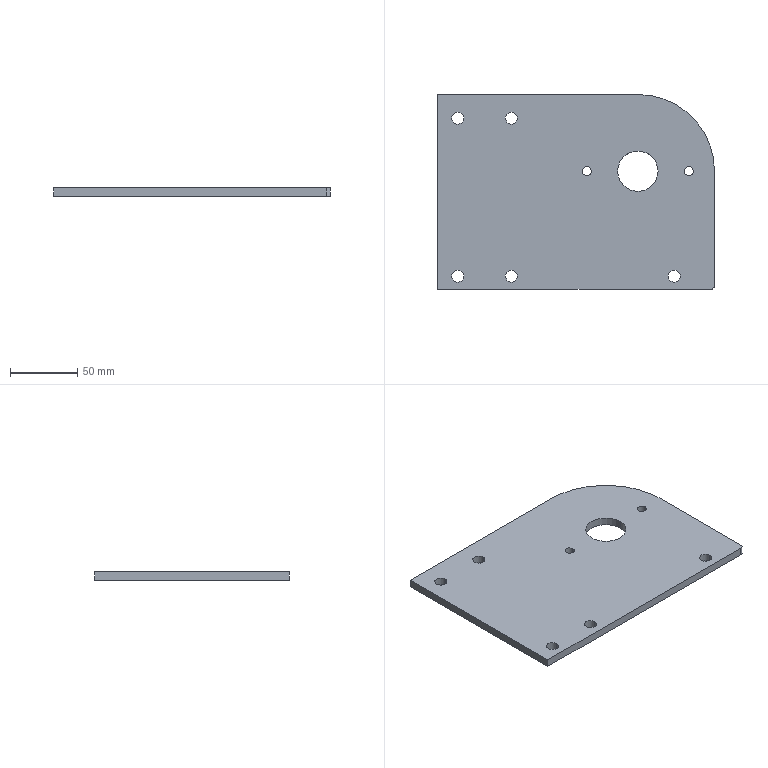Part | SolidWorks | features ICE 6, Fillet 5, HoleWzd 2, CirPattern 1, Extrusion 1 | 1 solid | 24 faces | box 206 x 145 x 6 mm | volume 168439 mm3 | cylinder 18 | plane 6 | commonest cylinder face diameters 9 x10 6.8 x4 30 x2 6 x1 114 x1
STEP:
#1=CARTESIAN_POINT('',(68.5,-62.5,0.));
#2=VERTEX_POINT('',#1);
#3=CARTESIAN_POINT('',(77.5,-62.5,0.));
#4=VERTEX_POINT('',#3);
#5=CARTESIAN_POINT('',(73.,-62.5,0.));
#6=DIRECTION('',(0.,0.,1.));
#7=DIRECTION('',(1.,0.,0.));
#8=AXIS2_PLACEMENT_3D('',#5,#6,#7);
#9=CIRCLE('',#8,4.5);
#10=EDGE_CURVE('',#2,#4,#9,.T.);
#11=ORIENTED_EDGE('',*,*,#10,.F.);
#12=CARTESIAN_POINT('',(68.5,-62.5,6.));
#13=VERTEX_POINT('',#12);
#14=CARTESIAN_POINT('',(68.5,-62.5,0.));
#15=DIRECTION('',(0.,0.,1.));
#16=VECTOR('',#15,1000.);
#17=LINE('',#14,#16);
#18=EDGE_CURVE('',#2,#13,#17,.T.);
#19=ORIENTED_EDGE('',*,*,#18,.T.);
#20=CARTESIAN_POINT('',(77.5,-62.5,6.));
#21=VERTEX_POINT('',#20);
#22=CARTESIAN_POINT('',(73.,-62.5,6.));
#23=DIRECTION('',(0.,0.,1.));
#24=DIRECTION('',(1.,0.,0.));
#25=AXIS2_PLACEMENT_3D('',#22,#23,#24);
#26=CIRCLE('',#25,4.5);
#27=EDGE_CURVE('',#13,#21,#26,.T.);
#28=ORIENTED_EDGE('',*,*,#27,.T.);
#29=CARTESIAN_POINT('',(77.5,-62.5,0.));
#30=DIRECTION('',(0.,0.,1.));
#31=VECTOR('',#30,1000.);
#32=LINE('',#29,#31);
#33=EDGE_CURVE('',#4,#21,#32,.T.);
#34=ORIENTED_EDGE('',*,*,#33,.F.);
#35=EDGE_LOOP('',(#11,#19,#28,#34));
#36=FACE_OUTER_BOUND('',#35,.T.);
#37=CARTESIAN_POINT('',(73.,-62.5,0.));
#38=DIRECTION('',(0.,0.,1.));
#39=DIRECTION('',(1.,0.,0.));
#40=AXIS2_PLACEMENT_3D('',#37,#38,#39);
#41=CYLINDRICAL_SURFACE('',#40,4.5);
#42=ADVANCED_FACE('',(#36),#41,.F.);
#43=CARTESIAN_POINT('',(80.6,15.5,0.));
#44=VERTEX_POINT('',#43);
#45=CARTESIAN_POINT('',(87.4,15.5,0.));
#46=VERTEX_POINT('',#45);
#47=CARTESIAN_POINT('',(84.,15.5,0.));
#48=DIRECTION('',(0.,0.,1.));
#49=DIRECTION('',(1.,0.,0.));
#50=AXIS2_PLACEMENT_3D('',#47,#48,#49);
#51=CIRCLE('',#50,3.4);
#52=EDGE_CURVE('',#44,#46,#51,.T.);
#53=ORIENTED_EDGE('',*,*,#52,.F.);
#54=CARTESIAN_POINT('',(80.6,15.5,6.));
#55=VERTEX_POINT('',#54);
#56=CARTESIAN_POINT('',(80.6,15.5,6.));
#57=DIRECTION('',(0.,0.,1.));
#58=VECTOR('',#57,1000.);
#59=LINE('',#56,#58);
#60=EDGE_CURVE('',#44,#55,#59,.T.);
#61=ORIENTED_EDGE('',*,*,#60,.T.);
#62=CARTESIAN_POINT('',(87.4,15.5,6.));
#63=VERTEX_POINT('',#62);
#64=CARTESIAN_POINT('',(84.,15.5,6.));
#65=DIRECTION('',(0.,0.,1.));
#66=DIRECTION('',(1.,0.,0.));
#67=AXIS2_PLACEMENT_3D('',#64,#65,#66);
#68=CIRCLE('',#67,3.4);
#69=EDGE_CURVE('',#55,#63,#68,.T.);
#70=ORIENTED_EDGE('',*,*,#69,.T.);
#71=CARTESIAN_POINT('',(87.4,15.5,6.));
#72=DIRECTION('',(0.,0.,1.));
#73=VECTOR('',#72,1000.);
#74=LINE('',#71,#73);
#75=EDGE_CURVE('',#46,#63,#74,.T.);
#76=ORIENTED_EDGE('',*,*,#75,.F.);
#77=EDGE_LOOP('',(#53,#61,#70,#76));
#78=FACE_OUTER_BOUND('',#77,.T.);
#79=CARTESIAN_POINT('',(84.,15.5,6.));
#80=DIRECTION('',(0.,0.,1.));
#81=DIRECTION('',(1.,0.,0.));
#82=AXIS2_PLACEMENT_3D('',#79,#80,#81);
#83=CYLINDRICAL_SURFACE('',#82,3.4);
#84=ADVANCED_FACE('',(#78),#83,.F.);
#85=CARTESIAN_POINT('',(4.6,15.5,0.));
#86=VERTEX_POINT('',#85);
#87=CARTESIAN_POINT('',(11.4,15.5,0.));
#88=VERTEX_POINT('',#87);
#89=CARTESIAN_POINT('',(8.,15.5,0.));
#90=DIRECTION('',(0.,0.,1.));
#91=DIRECTION('',(1.,0.,0.));
#92=AXIS2_PLACEMENT_3D('',#89,#90,#91);
#93=CIRCLE('',#92,3.4);
#94=EDGE_CURVE('',#86,#88,#93,.T.);
#95=ORIENTED_EDGE('',*,*,#94,.F.);
#96=CARTESIAN_POINT('',(4.6,15.5,6.));
#97=VERTEX_POINT('',#96);
#98=CARTESIAN_POINT('',(4.6,15.5,6.));
#99=DIRECTION('',(0.,0.,1.));
#100=VECTOR('',#99,1000.);
#101=LINE('',#98,#100);
#102=EDGE_CURVE('',#86,#97,#101,.T.);
#103=ORIENTED_EDGE('',*,*,#102,.T.);
#104=CARTESIAN_POINT('',(11.4,15.5,6.));
#105=VERTEX_POINT('',#104);
#106=CARTESIAN_POINT('',(8.,15.5,6.));
#107=DIRECTION('',(0.,0.,1.));
#108=DIRECTION('',(1.,0.,0.));
#109=AXIS2_PLACEMENT_3D('',#106,#107,#108);
#110=CIRCLE('',#109,3.4);
#111=EDGE_CURVE('',#97,#105,#110,.T.);
#112=ORIENTED_EDGE('',*,*,#111,.T.);
#113=CARTESIAN_POINT('',(11.4,15.5,6.));
#114=DIRECTION('',(0.,0.,1.));
#115=VECTOR('',#114,1000.);
#116=LINE('',#113,#115);
#117=EDGE_CURVE('',#88,#105,#116,.T.);
#118=ORIENTED_EDGE('',*,*,#117,.F.);
#119=EDGE_LOOP('',(#95,#103,#112,#118));
#120=FACE_OUTER_BOUND('',#119,.T.);
#121=CARTESIAN_POINT('',(8.,15.5,6.));
#122=DIRECTION('',(0.,0.,1.));
#123=DIRECTION('',(1.,0.,0.));
#124=AXIS2_PLACEMENT_3D('',#121,#122,#123);
#125=CYLINDRICAL_SURFACE('',#124,3.4);
#126=ADVANCED_FACE('',(#120),#125,.F.);
#127=CARTESIAN_POINT('',(31.,15.5,0.));
#128=VERTEX_POINT('',#127);
#129=CARTESIAN_POINT('',(61.,15.5,0.));
#130=VERTEX_POINT('',#129);
#131=CARTESIAN_POINT('',(46.,15.5,0.));
#132=DIRECTION('',(0.,0.,1.));
#133=DIRECTION('',(1.,0.,0.));
#134=AXIS2_PLACEMENT_3D('',#131,#132,#133);
#135=CIRCLE('',#134,15.);
#136=EDGE_CURVE('',#128,#130,#135,.T.);
#137=ORIENTED_EDGE('',*,*,#136,.F.);
#138=CARTESIAN_POINT('',(31.,15.5,6.));
#139=VERTEX_POINT('',#138);
#140=CARTESIAN_POINT('',(31.,15.5,0.));
#141=DIRECTION('',(0.,0.,1.));
#142=VECTOR('',#141,1000.);
#143=LINE('',#140,#142);
#144=EDGE_CURVE('',#128,#139,#143,.T.);
#145=ORIENTED_EDGE('',*,*,#144,.T.);
#146=CARTESIAN_POINT('',(61.,15.5,6.));
#147=VERTEX_POINT('',#146);
#148=CARTESIAN_POINT('',(46.,15.5,6.));
#149=DIRECTION('',(0.,0.,1.));
#150=DIRECTION('',(1.,0.,0.));
#151=AXIS2_PLACEMENT_3D('',#148,#149,#150);
#152=CIRCLE('',#151,15.);
#153=EDGE_CURVE('',#139,#147,#152,.T.);
#154=ORIENTED_EDGE('',*,*,#153,.T.);
#155=CARTESIAN_POINT('',(61.,15.5,0.));
#156=DIRECTION('',(0.,0.,1.));
#157=VECTOR('',#156,1000.);
#158=LINE('',#155,#157);
#159=EDGE_CURVE('',#130,#147,#158,.T.);
#160=ORIENTED_EDGE('',*,*,#159,.F.);
#161=EDGE_LOOP('',(#137,#145,#154,#160));
#162=FACE_OUTER_BOUND('',#161,.T.);
#163=CARTESIAN_POINT('',(46.,15.5,0.));
#164=DIRECTION('',(0.,0.,1.));
#165=DIRECTION('',(1.,0.,0.));
#166=AXIS2_PLACEMENT_3D('',#163,#164,#165);
#167=CYLINDRICAL_SURFACE('',#166,15.);
#168=ADVANCED_FACE('',(#162),#167,.F.);
#169=CARTESIAN_POINT('',(-52.5,-62.5,0.));
#170=VERTEX_POINT('',#169);
#171=CARTESIAN_POINT('',(-43.5,-62.5,0.));
#172=VERTEX_POINT('',#171);
#173=CARTESIAN_POINT('',(-48.,-62.5,0.));
#174=DIRECTION('',(0.,0.,1.));
#175=DIRECTION('',(1.,0.,0.));
#176=AXIS2_PLACEMENT_3D('',#173,#174,#175);
#177=CIRCLE('',#176,4.5);
#178=EDGE_CURVE('',#170,#172,#177,.T.);
#179=ORIENTED_EDGE('',*,*,#178,.F.);
#180=CARTESIAN_POINT('',(-52.5,-62.5,6.));
#181=VERTEX_POINT('',#180);
#182=CARTESIAN_POINT('',(-52.5,-62.5,0.));
#183=DIRECTION('',(0.,0.,1.));
#184=VECTOR('',#183,1000.);
#185=LINE('',#182,#184);
#186=EDGE_CURVE('',#170,#181,#185,.T.);
#187=ORIENTED_EDGE('',*,*,#186,.T.);
#188=CARTESIAN_POINT('',(-43.5,-62.5,6.));
#189=VERTEX_POINT('',#188);
#190=CARTESIAN_POINT('',(-48.,-62.5,6.));
#191=DIRECTION('',(0.,0.,1.));
#192=DIRECTION('',(1.,0.,0.));
#193=AXIS2_PLACEMENT_3D('',#190,#191,#192);
#194=CIRCLE('',#193,4.5);
#195=EDGE_CURVE('',#181,#189,#194,.T.);
#196=ORIENTED_EDGE('',*,*,#195,.T.);
#197=CARTESIAN_POINT('',(-43.5,-62.5,0.));
#198=DIRECTION('',(0.,0.,1.));
#199=VECTOR('',#198,1000.);
#200=LINE('',#197,#199);
#201=EDGE_CURVE('',#172,#189,#200,.T.);
#202=ORIENTED_EDGE('',*,*,#201,.F.);
#203=EDGE_LOOP('',(#179,#187,#196,#202));
#204=FACE_OUTER_BOUND('',#203,.T.);
#205=CARTESIAN_POINT('',(-48.,-62.5,0.));
#206=DIRECTION('',(0.,0.,1.));
#207=DIRECTION('',(1.,0.,0.));
#208=AXIS2_PLACEMENT_3D('',#205,#206,#207);
#209=CYLINDRICAL_SURFACE('',#208,4.5);
#210=ADVANCED_FACE('',(#204),#209,.F.);
#211=CARTESIAN_POINT('',(-92.5,-62.5,0.));
#212=VERTEX_POINT('',#211);
#213=CARTESIAN_POINT('',(-83.5,-62.5,0.));
#214=VERTEX_POINT('',#213);
#215=CARTESIAN_POINT('',(-88.,-62.5,0.));
#216=DIRECTION('',(0.,0.,1.));
#217=DIRECTION('',(1.,0.,0.));
#218=AXIS2_PLACEMENT_3D('',#215,#216,#217);
#219=CIRCLE('',#218,4.5);
#220=EDGE_CURVE('',#212,#214,#219,.T.);
#221=ORIENTED_EDGE('',*,*,#220,.F.);
#222=CARTESIAN_POINT('',(-92.5,-62.5,6.));
#223=VERTEX_POINT('',#222);
#224=CARTESIAN_POINT('',(-92.5,-62.5,0.));
#225=DIRECTION('',(0.,0.,1.));
#226=VECTOR('',#225,1000.);
#227=LINE('',#224,#226);
#228=EDGE_CURVE('',#212,#223,#227,.T.);
#229=ORIENTED_EDGE('',*,*,#228,.T.);
#230=CARTESIAN_POINT('',(-83.5,-62.5,6.));
#231=VERTEX_POINT('',#230);
#232=CARTESIAN_POINT('',(-88.,-62.5,6.));
#233=DIRECTION('',(0.,0.,1.));
#234=DIRECTION('',(1.,0.,0.));
#235=AXIS2_PLACEMENT_3D('',#232,#233,#234);
#236=CIRCLE('',#235,4.5);
#237=EDGE_CURVE('',#223,#231,#236,.T.);
#238=ORIENTED_EDGE('',*,*,#237,.T.);
#239=CARTESIAN_POINT('',(-83.5,-62.5,0.));
#240=DIRECTION('',(0.,0.,1.));
#241=VECTOR('',#240,1000.);
#242=LINE('',#239,#241);
#243=EDGE_CURVE('',#214,#231,#242,.T.);
#244=ORIENTED_EDGE('',*,*,#243,.F.);
#245=EDGE_LOOP('',(#221,#229,#238,#244));
#246=FACE_OUTER_BOUND('',#245,.T.);
#247=CARTESIAN_POINT('',(-88.,-62.5,0.));
#248=DIRECTION('',(0.,0.,1.));
#249=DIRECTION('',(1.,0.,0.));
#250=AXIS2_PLACEMENT_3D('',#247,#248,#249);
#251=CYLINDRICAL_SURFACE('',#250,4.5);
#252=ADVANCED_FACE('',(#246),#251,.F.);
#253=CARTESIAN_POINT('',(-52.5,55.,0.));
#254=VERTEX_POINT('',#253);
#255=CARTESIAN_POINT('',(-43.5,55.,0.));
#256=VERTEX_POINT('',#255);
#257=CARTESIAN_POINT('',(-48.,55.,0.));
#258=DIRECTION('',(0.,0.,1.));
#259=DIRECTION('',(1.,0.,0.));
#260=AXIS2_PLACEMENT_3D('',#257,#258,#259);
#261=CIRCLE('',#260,4.5);
#262=EDGE_CURVE('',#254,#256,#261,.T.);
#263=ORIENTED_EDGE('',*,*,#262,.F.);
#264=CARTESIAN_POINT('',(-52.5,55.,6.));
#265=VERTEX_POINT('',#264);
#266=CARTESIAN_POINT('',(-52.5,55.,0.));
#267=DIRECTION('',(0.,0.,1.));
#268=VECTOR('',#267,1000.);
#269=LINE('',#266,#268);
#270=EDGE_CURVE('',#254,#265,#269,.T.);
#271=ORIENTED_EDGE('',*,*,#270,.T.);
#272=CARTESIAN_POINT('',(-43.5,55.,6.));
#273=VERTEX_POINT('',#272);
#274=CARTESIAN_POINT('',(-48.,55.,6.));
#275=DIRECTION('',(0.,0.,1.));
#276=DIRECTION('',(1.,0.,0.));
#277=AXIS2_PLACEMENT_3D('',#274,#275,#276);
#278=CIRCLE('',#277,4.5);
#279=EDGE_CURVE('',#265,#273,#278,.T.);
#280=ORIENTED_EDGE('',*,*,#279,.T.);
#281=CARTESIAN_POINT('',(-43.5,55.,0.));
#282=DIRECTION('',(0.,0.,1.));
#283=VECTOR('',#282,1000.);
#284=LINE('',#281,#283);
#285=EDGE_CURVE('',#256,#273,#284,.T.);
#286=ORIENTED_EDGE('',*,*,#285,.F.);
#287=EDGE_LOOP('',(#263,#271,#280,#286));
#288=FACE_OUTER_BOUND('',#287,.T.);
#289=CARTESIAN_POINT('',(-48.,55.,0.));
#290=DIRECTION('',(0.,0.,1.));
#291=DIRECTION('',(1.,0.,0.));
#292=AXIS2_PLACEMENT_3D('',#289,#290,#291);
#293=CYLINDRICAL_SURFACE('',#292,4.5);
#294=ADVANCED_FACE('',(#288),#293,.F.);
#295=CARTESIAN_POINT('',(-92.5,55.,0.));
#296=VERTEX_POINT('',#295);
#297=CARTESIAN_POINT('',(-83.5,55.,0.));
#298=VERTEX_POINT('',#297);
#299=CARTESIAN_POINT('',(-88.,55.,0.));
#300=DIRECTION('',(0.,0.,1.));
#301=DIRECTION('',(1.,0.,0.));
#302=AXIS2_PLACEMENT_3D('',#299,#300,#301);
#303=CIRCLE('',#302,4.5);
#304=EDGE_CURVE('',#296,#298,#303,.T.);
#305=ORIENTED_EDGE('',*,*,#304,.F.);
#306=CARTESIAN_POINT('',(-92.5,55.,6.));
#307=VERTEX_POINT('',#306);
#308=CARTESIAN_POINT('',(-92.5,55.,0.));
#309=DIRECTION('',(0.,0.,1.));
#310=VECTOR('',#309,1000.);
#311=LINE('',#308,#310);
#312=EDGE_CURVE('',#296,#307,#311,.T.);
#313=ORIENTED_EDGE('',*,*,#312,.T.);
#314=CARTESIAN_POINT('',(-83.5,55.,6.));
#315=VERTEX_POINT('',#314);
#316=CARTESIAN_POINT('',(-88.,55.,6.));
#317=DIRECTION('',(0.,0.,1.));
#318=DIRECTION('',(1.,0.,0.));
#319=AXIS2_PLACEMENT_3D('',#316,#317,#318);
#320=CIRCLE('',#319,4.5);
#321=EDGE_CURVE('',#307,#315,#320,.T.);
#322=ORIENTED_EDGE('',*,*,#321,.T.);
#323=CARTESIAN_POINT('',(-83.5,55.,0.));
#324=DIRECTION('',(0.,0.,1.));
#325=VECTOR('',#324,1000.);
#326=LINE('',#323,#325);
#327=EDGE_CURVE('',#298,#315,#326,.T.);
#328=ORIENTED_EDGE('',*,*,#327,.F.);
#329=EDGE_LOOP('',(#305,#313,#322,#328));
#330=FACE_OUTER_BOUND('',#329,.T.);
#331=CARTESIAN_POINT('',(-88.,55.,0.));
#332=DIRECTION('',(0.,0.,1.));
#333=DIRECTION('',(1.,0.,0.));
#334=AXIS2_PLACEMENT_3D('',#331,#332,#333);
#335=CYLINDRICAL_SURFACE('',#334,4.5);
#336=ADVANCED_FACE('',(#330),#335,.F.);
#337=CARTESIAN_POINT('',(-103.,72.5,0.));
#338=VERTEX_POINT('',#337);
#339=CARTESIAN_POINT('',(-103.,-72.5,0.));
#340=VERTEX_POINT('',#339);
#341=CARTESIAN_POINT('',(-103.,72.5,0.));
#342=DIRECTION('',(0.,-1.,0.));
#343=VECTOR('',#342,1000.);
#344=LINE('',#341,#343);
#345=EDGE_CURVE('',#338,#340,#344,.T.);
#346=ORIENTED_EDGE('',*,*,#345,.T.);
#347=CARTESIAN_POINT('',(-103.,-72.5,6.));
#348=VERTEX_POINT('',#347);
#349=CARTESIAN_POINT('',(-103.,-72.5,6.));
#350=DIRECTION('',(0.,0.,-1.));
#351=VECTOR('',#350,1000.);
#352=LINE('',#349,#351);
#353=EDGE_CURVE('',#348,#340,#352,.T.);
#354=ORIENTED_EDGE('',*,*,#353,.F.);
#355=CARTESIAN_POINT('',(-103.,72.5,6.));
#356=VERTEX_POINT('',#355);
#357=CARTESIAN_POINT('',(-103.,72.5,6.));
#358=DIRECTION('',(0.,-1.,0.));
#359=VECTOR('',#358,1000.);
#360=LINE('',#357,#359);
#361=EDGE_CURVE('',#356,#348,#360,.T.);
#362=ORIENTED_EDGE('',*,*,#361,.F.);
#363=CARTESIAN_POINT('',(-103.,72.5,6.));
#364=DIRECTION('',(0.,0.,-1.));
#365=VECTOR('',#364,1000.);
#366=LINE('',#363,#365);
#367=EDGE_CURVE('',#356,#338,#366,.T.);
#368=ORIENTED_EDGE('',*,*,#367,.T.);
#369=EDGE_LOOP('',(#346,#354,#362,#368));
#370=FACE_OUTER_BOUND('',#369,.T.);
#371=CARTESIAN_POINT('',(-103.,72.5,6.));
#372=DIRECTION('',(1.,0.,0.));
#373=DIRECTION('',(0.,0.,-1.));
#374=AXIS2_PLACEMENT_3D('',#371,#372,#373);
#375=PLANE('',#374);
#376=ADVANCED_FACE('',(#370),#375,.F.);
#377=CARTESIAN_POINT('',(100.,-72.5,0.));
#378=VERTEX_POINT('',#377);
#379=CARTESIAN_POINT('',(-103.,-72.5,0.));
#380=DIRECTION('',(1.,0.,0.));
#381=VECTOR('',#380,1000.);
#382=LINE('',#379,#381);
#383=EDGE_CURVE('',#340,#378,#382,.T.);
#384=ORIENTED_EDGE('',*,*,#383,.T.);
#385=CARTESIAN_POINT('',(100.,-72.5,6.));
#386=VERTEX_POINT('',#385);
#387=CARTESIAN_POINT('',(100.,-72.5,6.));
#388=DIRECTION('',(0.,0.,1.));
#389=VECTOR('',#388,1000.);
#390=LINE('',#387,#389);
#391=EDGE_CURVE('',#378,#386,#390,.T.);
#392=ORIENTED_EDGE('',*,*,#391,.T.);
#393=CARTESIAN_POINT('',(-103.,-72.5,6.));
#394=DIRECTION('',(1.,0.,0.));
#395=VECTOR('',#394,1000.);
#396=LINE('',#393,#395);
#397=EDGE_CURVE('',#348,#386,#396,.T.);
#398=ORIENTED_EDGE('',*,*,#397,.F.);
#399=ORIENTED_EDGE('',*,*,#353,.T.);
#400=EDGE_LOOP('',(#384,#392,#398,#399));
#401=FACE_OUTER_BOUND('',#400,.T.);
#402=CARTESIAN_POINT('',(-103.,-72.5,6.));
#403=DIRECTION('',(0.,1.,0.));
#404=DIRECTION('',(0.,0.,1.));
#405=AXIS2_PLACEMENT_3D('',#402,#403,#404);
#406=PLANE('',#405);
#407=ADVANCED_FACE('',(#401),#406,.F.);
#408=CARTESIAN_POINT('',(103.,-69.5,6.));
#409=VERTEX_POINT('',#408);
#410=CARTESIAN_POINT('',(103.,15.5,6.));
#411=VERTEX_POINT('',#410);
#412=CARTESIAN_POINT('',(103.,72.5,6.));
#413=DIRECTION('',(0.,1.,0.));
#414=VECTOR('',#413,1000.);
#415=LINE('',#412,#414);
#416=EDGE_CURVE('',#409,#411,#415,.T.);
#417=ORIENTED_EDGE('',*,*,#416,.F.);
#418=CARTESIAN_POINT('',(103.,-69.5,0.));
#419=VERTEX_POINT('',#418);
#420=CARTESIAN_POINT('',(103.,-69.5,6.));
#421=DIRECTION('',(0.,0.,-1.));
#422=VECTOR('',#421,1000.);
#423=LINE('',#420,#422);
#424=EDGE_CURVE('',#409,#419,#423,.T.);
#425=ORIENTED_EDGE('',*,*,#424,.T.);
#426=CARTESIAN_POINT('',(103.,15.5,0.));
#427=VERTEX_POINT('',#426);
#428=CARTESIAN_POINT('',(103.,72.5,0.));
#429=DIRECTION('',(0.,1.,0.));
#430=VECTOR('',#429,1000.);
#431=LINE('',#428,#430);
#432=EDGE_CURVE('',#419,#427,#431,.T.);
#433=ORIENTED_EDGE('',*,*,#432,.T.);
#434=CARTESIAN_POINT('',(103.,15.5,6.));
#435=DIRECTION('',(0.,0.,1.));
#436=VECTOR('',#435,1000.);
#437=LINE('',#434,#436);
#438=EDGE_CURVE('',#427,#411,#437,.T.);
#439=ORIENTED_EDGE('',*,*,#438,.T.);
#440=EDGE_LOOP('',(#417,#425,#433,#439));
#441=FACE_OUTER_BOUND('',#440,.T.);
#442=CARTESIAN_POINT('',(103.,72.5,6.));
#443=DIRECTION('',(-1.,0.,0.));
#444=DIRECTION('',(0.,0.,1.));
#445=AXIS2_PLACEMENT_3D('',#442,#443,#444);
#446=PLANE('',#445);
#447=ADVANCED_FACE('',(#441),#446,.F.);
#448=CARTESIAN_POINT('',(46.,72.5,6.));
#449=VERTEX_POINT('',#448);
#450=CARTESIAN_POINT('',(-103.,72.5,6.));
#451=DIRECTION('',(-1.,0.,0.));
#452=VECTOR('',#451,1000.);
#453=LINE('',#450,#452);
#454=EDGE_CURVE('',#449,#356,#453,.T.);
#455=ORIENTED_EDGE('',*,*,#454,.F.);
#456=CARTESIAN_POINT('',(46.,72.5,0.));
#457=VERTEX_POINT('',#456);
#458=CARTESIAN_POINT('',(46.,72.5,6.));
#459=DIRECTION('',(0.,0.,-1.));
#460=VECTOR('',#459,1000.);
#461=LINE('',#458,#460);
#462=EDGE_CURVE('',#449,#457,#461,.T.);
#463=ORIENTED_EDGE('',*,*,#462,.T.);
#464=CARTESIAN_POINT('',(-103.,72.5,0.));
#465=DIRECTION('',(-1.,0.,0.));
#466=VECTOR('',#465,1000.);
#467=LINE('',#464,#466);
#468=EDGE_CURVE('',#457,#338,#467,.T.);
#469=ORIENTED_EDGE('',*,*,#468,.T.);
#470=ORIENTED_EDGE('',*,*,#367,.F.);
#471=EDGE_LOOP('',(#455,#463,#469,#470));
#472=FACE_OUTER_BOUND('',#471,.T.);
#473=CARTESIAN_POINT('',(-103.,72.5,6.));
#474=DIRECTION('',(0.,-1.,0.));
#475=DIRECTION('',(0.,0.,-1.));
#476=AXIS2_PLACEMENT_3D('',#473,#474,#475);
#477=PLANE('',#476);
#478=ADVANCED_FACE('',(#472),#477,.F.);
#479=CARTESIAN_POINT('',(73.,-62.5,6.));
#480=DIRECTION('',(0.,0.,1.));
#481=DIRECTION('',(1.,0.,0.));
#482=AXIS2_PLACEMENT_3D('',#479,#480,#481);
#483=CIRCLE('',#482,4.5);
#484=EDGE_CURVE('',#21,#13,#483,.T.);
#485=ORIENTED_EDGE('',*,*,#484,.F.);
#486=ORIENTED_EDGE('',*,*,#27,.F.);
#487=EDGE_LOOP('',(#485,#486));
#488=FACE_BOUND('',#487,.T.);
#489=CARTESIAN_POINT('',(84.,15.5,6.));
#490=DIRECTION('',(0.,0.,1.));
#491=DIRECTION('',(1.,0.,0.));
#492=AXIS2_PLACEMENT_3D('',#489,#490,#491);
#493=CIRCLE('',#492,3.4);
#494=EDGE_CURVE('',#63,#55,#493,.T.);
#495=ORIENTED_EDGE('',*,*,#494,.F.);
#496=ORIENTED_EDGE('',*,*,#69,.F.);
#497=EDGE_LOOP('',(#495,#496));
#498=FACE_BOUND('',#497,.T.);
#499=CARTESIAN_POINT('',(8.,15.5,6.));
#500=DIRECTION('',(0.,0.,1.));
#501=DIRECTION('',(1.,0.,0.));
#502=AXIS2_PLACEMENT_3D('',#499,#500,#501);
#503=CIRCLE('',#502,3.4);
#504=EDGE_CURVE('',#105,#97,#503,.T.);
#505=ORIENTED_EDGE('',*,*,#504,.F.);
#506=ORIENTED_EDGE('',*,*,#111,.F.);
#507=EDGE_LOOP('',(#505,#506));
#508=FACE_BOUND('',#507,.T.);
#509=CARTESIAN_POINT('',(46.,15.5,6.));
#510=DIRECTION('',(0.,0.,1.));
#511=DIRECTION('',(1.,0.,0.));
#512=AXIS2_PLACEMENT_3D('',#509,#510,#511);
#513=CIRCLE('',#512,15.);
#514=EDGE_CURVE('',#147,#139,#513,.T.);
#515=ORIENTED_EDGE('',*,*,#514,.F.);
#516=ORIENTED_EDGE('',*,*,#153,.F.);
#517=EDGE_LOOP('',(#515,#516));
#518=FACE_BOUND('',#517,.T.);
#519=CARTESIAN_POINT('',(-48.,-62.5,6.));
#520=DIRECTION('',(0.,0.,1.));
#521=DIRECTION('',(1.,0.,0.));
#522=AXIS2_PLACEMENT_3D('',#519,#520,#521);
#523=CIRCLE('',#522,4.5);
#524=EDGE_CURVE('',#189,#181,#523,.T.);
#525=ORIENTED_EDGE('',*,*,#524,.F.);
#526=ORIENTED_EDGE('',*,*,#195,.F.);
#527=EDGE_LOOP('',(#525,#526));
#528=FACE_BOUND('',#527,.T.);
#529=CARTESIAN_POINT('',(-88.,-62.5,6.));
#530=DIRECTION('',(0.,0.,1.));
#531=DIRECTION('',(1.,0.,0.));
#532=AXIS2_PLACEMENT_3D('',#529,#530,#531);
#533=CIRCLE('',#532,4.5);
#534=EDGE_CURVE('',#231,#223,#533,.T.);
#535=ORIENTED_EDGE('',*,*,#534,.F.);
#536=ORIENTED_EDGE('',*,*,#237,.F.);
#537=EDGE_LOOP('',(#535,#536));
#538=FACE_BOUND('',#537,.T.);
#539=CARTESIAN_POINT('',(-48.,55.,6.));
#540=DIRECTION('',(0.,0.,1.));
#541=DIRECTION('',(1.,0.,0.));
#542=AXIS2_PLACEMENT_3D('',#539,#540,#541);
#543=CIRCLE('',#542,4.5);
#544=EDGE_CURVE('',#273,#265,#543,.T.);
#545=ORIENTED_EDGE('',*,*,#544,.F.);
#546=ORIENTED_EDGE('',*,*,#279,.F.);
#547=EDGE_LOOP('',(#545,#546));
#548=FACE_BOUND('',#547,.T.);
#549=CARTESIAN_POINT('',(-88.,55.,6.));
#550=DIRECTION('',(0.,0.,1.));
#551=DIRECTION('',(1.,0.,0.));
#552=AXIS2_PLACEMENT_3D('',#549,#550,#551);
#553=CIRCLE('',#552,4.5);
#554=EDGE_CURVE('',#315,#307,#553,.T.);
#555=ORIENTED_EDGE('',*,*,#554,.F.);
#556=ORIENTED_EDGE('',*,*,#321,.F.);
#557=EDGE_LOOP('',(#555,#556));
#558=FACE_BOUND('',#557,.T.);
#559=ORIENTED_EDGE('',*,*,#397,.T.);
#560=CARTESIAN_POINT('',(100.,-69.5,6.));
#561=DIRECTION('',(0.,0.,1.));
#562=DIRECTION('',(1.,0.,0.));
#563=AXIS2_PLACEMENT_3D('',#560,#561,#562);
#564=CIRCLE('',#563,3.);
#565=EDGE_CURVE('',#386,#409,#564,.T.);
#566=ORIENTED_EDGE('',*,*,#565,.T.);
#567=ORIENTED_EDGE('',*,*,#416,.T.);
#568=CARTESIAN_POINT('',(46.,15.5,6.));
#569=DIRECTION('',(0.,0.,1.));
#570=DIRECTION('',(1.,0.,0.));
#571=AXIS2_PLACEMENT_3D('',#568,#569,#570);
#572=CIRCLE('',#571,57.);
#573=EDGE_CURVE('',#411,#449,#572,.T.);
#574=ORIENTED_EDGE('',*,*,#573,.T.);
#575=ORIENTED_EDGE('',*,*,#454,.T.);
#576=ORIENTED_EDGE('',*,*,#361,.T.);
#577=EDGE_LOOP('',(#559,#566,#567,#574,#575,#576));
#578=FACE_OUTER_BOUND('',#577,.T.);
#579=CARTESIAN_POINT('',(0.,0.,6.));
#580=DIRECTION('',(0.,0.,1.));
#581=DIRECTION('',(1.,0.,0.));
#582=AXIS2_PLACEMENT_3D('',#579,#580,#581);
#583=PLANE('',#582);
#584=ADVANCED_FACE('',(#488,#498,#508,#518,#528,#538,#548,#558,#578),#583,.T.);
#585=CARTESIAN_POINT('',(73.,-62.5,0.));
#586=DIRECTION('',(0.,0.,1.));
#587=DIRECTION('',(1.,0.,0.));
#588=AXIS2_PLACEMENT_3D('',#585,#586,#587);
#589=CIRCLE('',#588,4.5);
#590=EDGE_CURVE('',#4,#2,#589,.T.);
#591=ORIENTED_EDGE('',*,*,#590,.T.);
#592=ORIENTED_EDGE('',*,*,#10,.T.);
#593=EDGE_LOOP('',(#591,#592));
#594=FACE_BOUND('',#593,.T.);
#595=CARTESIAN_POINT('',(84.,15.5,0.));
#596=DIRECTION('',(0.,0.,1.));
#597=DIRECTION('',(1.,0.,0.));
#598=AXIS2_PLACEMENT_3D('',#595,#596,#597);
#599=CIRCLE('',#598,3.4);
#600=EDGE_CURVE('',#46,#44,#599,.T.);
#601=ORIENTED_EDGE('',*,*,#600,.T.);
#602=ORIENTED_EDGE('',*,*,#52,.T.);
#603=EDGE_LOOP('',(#601,#602));
#604=FACE_BOUND('',#603,.T.);
#605=CARTESIAN_POINT('',(8.,15.5,0.));
#606=DIRECTION('',(0.,0.,1.));
#607=DIRECTION('',(1.,0.,0.));
#608=AXIS2_PLACEMENT_3D('',#605,#606,#607);
#609=CIRCLE('',#608,3.4);
#610=EDGE_CURVE('',#88,#86,#609,.T.);
#611=ORIENTED_EDGE('',*,*,#610,.T.);
#612=ORIENTED_EDGE('',*,*,#94,.T.);
#613=EDGE_LOOP('',(#611,#612));
#614=FACE_BOUND('',#613,.T.);
#615=CARTESIAN_POINT('',(46.,15.5,0.));
#616=DIRECTION('',(0.,0.,1.));
#617=DIRECTION('',(1.,0.,0.));
#618=AXIS2_PLACEMENT_3D('',#615,#616,#617);
#619=CIRCLE('',#618,15.);
#620=EDGE_CURVE('',#130,#128,#619,.T.);
#621=ORIENTED_EDGE('',*,*,#620,.T.);
#622=ORIENTED_EDGE('',*,*,#136,.T.);
#623=EDGE_LOOP('',(#621,#622));
#624=FACE_BOUND('',#623,.T.);
#625=CARTESIAN_POINT('',(-48.,-62.5,0.));
#626=DIRECTION('',(0.,0.,1.));
#627=DIRECTION('',(1.,0.,0.));
#628=AXIS2_PLACEMENT_3D('',#625,#626,#627);
#629=CIRCLE('',#628,4.5);
#630=EDGE_CURVE('',#172,#170,#629,.T.);
#631=ORIENTED_EDGE('',*,*,#630,.T.);
#632=ORIENTED_EDGE('',*,*,#178,.T.);
#633=EDGE_LOOP('',(#631,#632));
#634=FACE_BOUND('',#633,.T.);
#635=CARTESIAN_POINT('',(-88.,-62.5,0.));
#636=DIRECTION('',(0.,0.,1.));
#637=DIRECTION('',(1.,0.,0.));
#638=AXIS2_PLACEMENT_3D('',#635,#636,#637);
#639=CIRCLE('',#638,4.5);
#640=EDGE_CURVE('',#214,#212,#639,.T.);
#641=ORIENTED_EDGE('',*,*,#640,.T.);
#642=ORIENTED_EDGE('',*,*,#220,.T.);
#643=EDGE_LOOP('',(#641,#642));
#644=FACE_BOUND('',#643,.T.);
#645=CARTESIAN_POINT('',(-48.,55.,0.));
#646=DIRECTION('',(0.,0.,1.));
#647=DIRECTION('',(1.,0.,0.));
#648=AXIS2_PLACEMENT_3D('',#645,#646,#647);
#649=CIRCLE('',#648,4.5);
#650=EDGE_CURVE('',#256,#254,#649,.T.);
#651=ORIENTED_EDGE('',*,*,#650,.T.);
#652=ORIENTED_EDGE('',*,*,#262,.T.);
#653=EDGE_LOOP('',(#651,#652));
#654=FACE_BOUND('',#653,.T.);
#655=CARTESIAN_POINT('',(-88.,55.,0.));
#656=DIRECTION('',(0.,0.,1.));
#657=DIRECTION('',(1.,0.,0.));
#658=AXIS2_PLACEMENT_3D('',#655,#656,#657);
#659=CIRCLE('',#658,4.5);
#660=EDGE_CURVE('',#298,#296,#659,.T.);
#661=ORIENTED_EDGE('',*,*,#660,.T.);
#662=ORIENTED_EDGE('',*,*,#304,.T.);
#663=EDGE_LOOP('',(#661,#662));
#664=FACE_BOUND('',#663,.T.);
#665=ORIENTED_EDGE('',*,*,#432,.F.);
#666=CARTESIAN_POINT('',(100.,-69.5,0.));
#667=DIRECTION('',(0.,0.,-1.));
#668=DIRECTION('',(1.,0.,0.));
#669=AXIS2_PLACEMENT_3D('',#666,#667,#668);
#670=CIRCLE('',#669,3.);
#671=EDGE_CURVE('',#419,#378,#670,.T.);
#672=ORIENTED_EDGE('',*,*,#671,.T.);
#673=ORIENTED_EDGE('',*,*,#383,.F.);
#674=ORIENTED_EDGE('',*,*,#345,.F.);
#675=ORIENTED_EDGE('',*,*,#468,.F.);
#676=CARTESIAN_POINT('',(46.,15.5,0.));
#677=DIRECTION('',(0.,0.,-1.));
#678=DIRECTION('',(1.,0.,0.));
#679=AXIS2_PLACEMENT_3D('',#676,#677,#678);
#680=CIRCLE('',#679,57.);
#681=EDGE_CURVE('',#457,#427,#680,.T.);
#682=ORIENTED_EDGE('',*,*,#681,.T.);
#683=EDGE_LOOP('',(#665,#672,#673,#674,#675,#682));
#684=FACE_OUTER_BOUND('',#683,.T.);
#685=CARTESIAN_POINT('',(0.,0.,0.));
#686=DIRECTION('',(0.,0.,1.));
#687=DIRECTION('',(1.,0.,0.));
#688=AXIS2_PLACEMENT_3D('',#685,#686,#687);
#689=PLANE('',#688);
#690=ADVANCED_FACE('',(#594,#604,#614,#624,#634,#644,#654,#664,#684),#689,.F.);
#691=ORIENTED_EDGE('',*,*,#312,.F.);
#692=ORIENTED_EDGE('',*,*,#660,.F.);
#693=ORIENTED_EDGE('',*,*,#327,.T.);
#694=ORIENTED_EDGE('',*,*,#554,.T.);
#695=EDGE_LOOP('',(#691,#692,#693,#694));
#696=FACE_OUTER_BOUND('',#695,.T.);
#697=CARTESIAN_POINT('',(-88.,55.,0.));
#698=DIRECTION('',(0.,0.,1.));
#699=DIRECTION('',(1.,0.,0.));
#700=AXIS2_PLACEMENT_3D('',#697,#698,#699);
#701=CYLINDRICAL_SURFACE('',#700,4.5);
#702=ADVANCED_FACE('',(#696),#701,.F.);
#703=ORIENTED_EDGE('',*,*,#270,.F.);
#704=ORIENTED_EDGE('',*,*,#650,.F.);
#705=ORIENTED_EDGE('',*,*,#285,.T.);
#706=ORIENTED_EDGE('',*,*,#544,.T.);
#707=EDGE_LOOP('',(#703,#704,#705,#706));
#708=FACE_OUTER_BOUND('',#707,.T.);
#709=CARTESIAN_POINT('',(-48.,55.,0.));
#710=DIRECTION('',(0.,0.,1.));
#711=DIRECTION('',(1.,0.,0.));
#712=AXIS2_PLACEMENT_3D('',#709,#710,#711);
#713=CYLINDRICAL_SURFACE('',#712,4.5);
#714=ADVANCED_FACE('',(#708),#713,.F.);
#715=ORIENTED_EDGE('',*,*,#228,.F.);
#716=ORIENTED_EDGE('',*,*,#640,.F.);
#717=ORIENTED_EDGE('',*,*,#243,.T.);
#718=ORIENTED_EDGE('',*,*,#534,.T.);
#719=EDGE_LOOP('',(#715,#716,#717,#718));
#720=FACE_OUTER_BOUND('',#719,.T.);
#721=CARTESIAN_POINT('',(-88.,-62.5,0.));
#722=DIRECTION('',(0.,0.,1.));
#723=DIRECTION('',(1.,0.,0.));
#724=AXIS2_PLACEMENT_3D('',#721,#722,#723);
#725=CYLINDRICAL_SURFACE('',#724,4.5);
#726=ADVANCED_FACE('',(#720),#725,.F.);
#727=ORIENTED_EDGE('',*,*,#186,.F.);
#728=ORIENTED_EDGE('',*,*,#630,.F.);
#729=ORIENTED_EDGE('',*,*,#201,.T.);
#730=ORIENTED_EDGE('',*,*,#524,.T.);
#731=EDGE_LOOP('',(#727,#728,#729,#730));
#732=FACE_OUTER_BOUND('',#731,.T.);
#733=CARTESIAN_POINT('',(-48.,-62.5,0.));
#734=DIRECTION('',(0.,0.,1.));
#735=DIRECTION('',(1.,0.,0.));
#736=AXIS2_PLACEMENT_3D('',#733,#734,#735);
#737=CYLINDRICAL_SURFACE('',#736,4.5);
#738=ADVANCED_FACE('',(#732),#737,.F.);
#739=ORIENTED_EDGE('',*,*,#144,.F.);
#740=ORIENTED_EDGE('',*,*,#620,.F.);
#741=ORIENTED_EDGE('',*,*,#159,.T.);
#742=ORIENTED_EDGE('',*,*,#514,.T.);
#743=EDGE_LOOP('',(#739,#740,#741,#742));
#744=FACE_OUTER_BOUND('',#743,.T.);
#745=CARTESIAN_POINT('',(46.,15.5,0.));
#746=DIRECTION('',(0.,0.,1.));
#747=DIRECTION('',(1.,0.,0.));
#748=AXIS2_PLACEMENT_3D('',#745,#746,#747);
#749=CYLINDRICAL_SURFACE('',#748,15.);
#750=ADVANCED_FACE('',(#744),#749,.F.);
#751=ORIENTED_EDGE('',*,*,#573,.F.);
#752=ORIENTED_EDGE('',*,*,#438,.F.);
#753=ORIENTED_EDGE('',*,*,#681,.F.);
#754=ORIENTED_EDGE('',*,*,#462,.F.);
#755=EDGE_LOOP('',(#751,#752,#753,#754));
#756=FACE_OUTER_BOUND('',#755,.T.);
#757=CARTESIAN_POINT('',(46.,15.5,6.));
#758=DIRECTION('',(0.,0.,-1.));
#759=DIRECTION('',(-1.,0.,0.));
#760=AXIS2_PLACEMENT_3D('',#757,#758,#759);
#761=CYLINDRICAL_SURFACE('',#760,57.);
#762=ADVANCED_FACE('',(#756),#761,.T.);
#763=ORIENTED_EDGE('',*,*,#102,.F.);
#764=ORIENTED_EDGE('',*,*,#610,.F.);
#765=ORIENTED_EDGE('',*,*,#117,.T.);
#766=ORIENTED_EDGE('',*,*,#504,.T.);
#767=EDGE_LOOP('',(#763,#764,#765,#766));
#768=FACE_OUTER_BOUND('',#767,.T.);
#769=CARTESIAN_POINT('',(8.,15.5,6.));
#770=DIRECTION('',(0.,0.,1.));
#771=DIRECTION('',(1.,0.,0.));
#772=AXIS2_PLACEMENT_3D('',#769,#770,#771);
#773=CYLINDRICAL_SURFACE('',#772,3.4);
#774=ADVANCED_FACE('',(#768),#773,.F.);
#775=ORIENTED_EDGE('',*,*,#60,.F.);
#776=ORIENTED_EDGE('',*,*,#600,.F.);
#777=ORIENTED_EDGE('',*,*,#75,.T.);
#778=ORIENTED_EDGE('',*,*,#494,.T.);
#779=EDGE_LOOP('',(#775,#776,#777,#778));
#780=FACE_OUTER_BOUND('',#779,.T.);
#781=CARTESIAN_POINT('',(84.,15.5,6.));
#782=DIRECTION('',(0.,0.,1.));
#783=DIRECTION('',(1.,0.,0.));
#784=AXIS2_PLACEMENT_3D('',#781,#782,#783);
#785=CYLINDRICAL_SURFACE('',#784,3.4);
#786=ADVANCED_FACE('',(#780),#785,.F.);
#787=ORIENTED_EDGE('',*,*,#18,.F.);
#788=ORIENTED_EDGE('',*,*,#590,.F.);
#789=ORIENTED_EDGE('',*,*,#33,.T.);
#790=ORIENTED_EDGE('',*,*,#484,.T.);
#791=EDGE_LOOP('',(#787,#788,#789,#790));
#792=FACE_OUTER_BOUND('',#791,.T.);
#793=CARTESIAN_POINT('',(73.,-62.5,0.));
#794=DIRECTION('',(0.,0.,1.));
#795=DIRECTION('',(1.,0.,0.));
#796=AXIS2_PLACEMENT_3D('',#793,#794,#795);
#797=CYLINDRICAL_SURFACE('',#796,4.5);
#798=ADVANCED_FACE('',(#792),#797,.F.);
#799=ORIENTED_EDGE('',*,*,#565,.F.);
#800=ORIENTED_EDGE('',*,*,#391,.F.);
#801=ORIENTED_EDGE('',*,*,#671,.F.);
#802=ORIENTED_EDGE('',*,*,#424,.F.);
#803=EDGE_LOOP('',(#799,#800,#801,#802));
#804=FACE_OUTER_BOUND('',#803,.T.);
#805=CARTESIAN_POINT('',(100.,-69.5,6.));
#806=DIRECTION('',(0.,0.,-1.));
#807=DIRECTION('',(-1.,0.,0.));
#808=AXIS2_PLACEMENT_3D('',#805,#806,#807);
#809=CYLINDRICAL_SURFACE('',#808,3.);
#810=ADVANCED_FACE('',(#804),#809,.T.);
#811=CLOSED_SHELL('',(#42,#84,#126,#168,#210,#252,#294,#336,#376,#407,#447,#478,#584,#690,#702,#714,#726,#738,#750,#762,#774,#786,#798,#810));
#812=MANIFOLD_SOLID_BREP('',#811);
#813=CARTESIAN_POINT('',(0.,0.,0.));
#814=DIRECTION('',(0.,0.,1.));
#815=DIRECTION('',(1.,0.,0.));
#816=AXIS2_PLACEMENT_3D('',#813,#814,#815);
#817=(LENGTH_UNIT()NAMED_UNIT(*)SI_UNIT(.MILLI.,.METRE.));
#818=UNCERTAINTY_MEASURE_WITH_UNIT(LENGTH_MEASURE(0.00001),#817,'','');
#819=(NAMED_UNIT(*)PLANE_ANGLE_UNIT()SI_UNIT($,.RADIAN.));
#820=(NAMED_UNIT(*)SI_UNIT($,.STERADIAN.)SOLID_ANGLE_UNIT());
#821=(GEOMETRIC_REPRESENTATION_CONTEXT(3)GLOBAL_UNCERTAINTY_ASSIGNED_CONTEXT((#818))GLOBAL_UNIT_ASSIGNED_CONTEXT((#817,#819,#820))REPRESENTATION_CONTEXT('',''));
#822=ADVANCED_BREP_SHAPE_REPRESENTATION('',(#812,#816),#821);